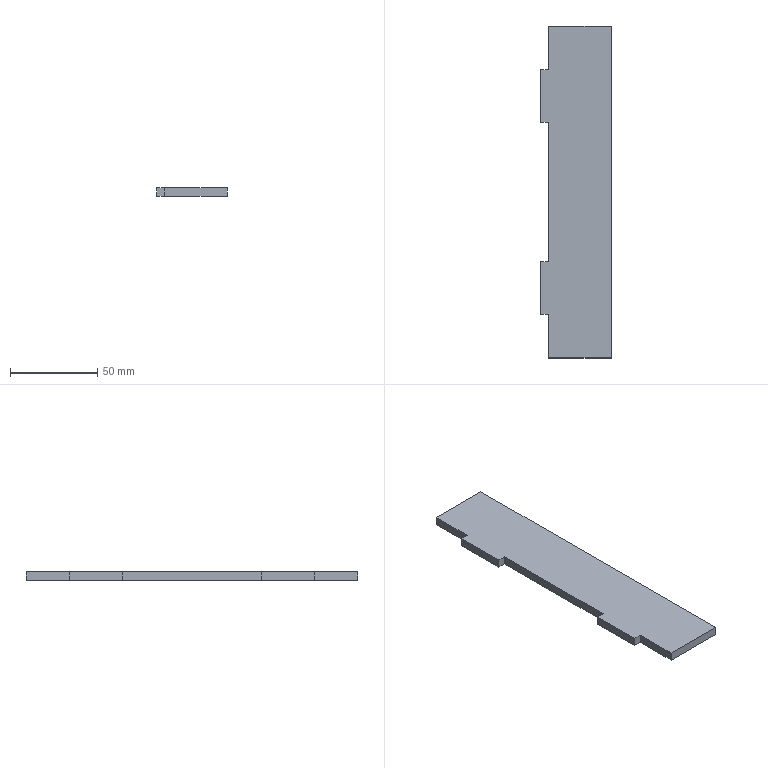Part | SolidWorks | features FlatPattern 1, SMBaseFlange 1, SheetMetal 1 | 1 solid | 14 faces | box 40.5 x 190 x 5 mm | volume 35550 mm3 | plane 14
STEP:
#1=CARTESIAN_POINT('',(-126.05,-77.454,0.));
#2=VERTEX_POINT('',#1);
#3=CARTESIAN_POINT('',(-126.05,-102.454,0.));
#4=VERTEX_POINT('',#3);
#5=CARTESIAN_POINT('',(-126.05,-102.454,0.));
#6=DIRECTION('',(0.,-1.,0.));
#7=VECTOR('',#6,1000.);
#8=LINE('',#5,#7);
#9=EDGE_CURVE('',#2,#4,#8,.T.);
#10=ORIENTED_EDGE('',*,*,#9,.F.);
#11=CARTESIAN_POINT('',(-126.05,-77.454,-5.));
#12=VERTEX_POINT('',#11);
#13=CARTESIAN_POINT('',(-126.05,-77.454,-5.));
#14=DIRECTION('',(0.,0.,1.));
#15=VECTOR('',#14,1000.);
#16=LINE('',#13,#15);
#17=EDGE_CURVE('',#12,#2,#16,.T.);
#18=ORIENTED_EDGE('',*,*,#17,.F.);
#19=CARTESIAN_POINT('',(-126.05,-102.454,-5.));
#20=VERTEX_POINT('',#19);
#21=CARTESIAN_POINT('',(-126.05,-102.454,-5.));
#22=DIRECTION('',(0.,-1.,0.));
#23=VECTOR('',#22,1000.);
#24=LINE('',#21,#23);
#25=EDGE_CURVE('',#12,#20,#24,.T.);
#26=ORIENTED_EDGE('',*,*,#25,.T.);
#27=CARTESIAN_POINT('',(-126.05,-102.454,-5.));
#28=DIRECTION('',(0.,0.,1.));
#29=VECTOR('',#28,1000.);
#30=LINE('',#27,#29);
#31=EDGE_CURVE('',#20,#4,#30,.T.);
#32=ORIENTED_EDGE('',*,*,#31,.T.);
#33=EDGE_LOOP('',(#10,#18,#26,#32));
#34=FACE_OUTER_BOUND('',#33,.T.);
#35=CARTESIAN_POINT('',(-126.05,-102.454,-5.));
#36=DIRECTION('',(-1.,0.,0.));
#37=DIRECTION('',(0.,0.,1.));
#38=AXIS2_PLACEMENT_3D('',#35,#36,#37);
#39=PLANE('',#38);
#40=ADVANCED_FACE('',(#34),#39,.T.);
#41=CARTESIAN_POINT('',(-130.55,-77.454,0.));
#42=VERTEX_POINT('',#41);
#43=CARTESIAN_POINT('',(-126.05,-77.454,0.));
#44=DIRECTION('',(1.,0.,0.));
#45=VECTOR('',#44,1000.);
#46=LINE('',#43,#45);
#47=EDGE_CURVE('',#42,#2,#46,.T.);
#48=ORIENTED_EDGE('',*,*,#47,.F.);
#49=CARTESIAN_POINT('',(-130.55,-77.454,-5.));
#50=VERTEX_POINT('',#49);
#51=CARTESIAN_POINT('',(-130.55,-77.454,-5.));
#52=DIRECTION('',(0.,0.,1.));
#53=VECTOR('',#52,1000.);
#54=LINE('',#51,#53);
#55=EDGE_CURVE('',#50,#42,#54,.T.);
#56=ORIENTED_EDGE('',*,*,#55,.F.);
#57=CARTESIAN_POINT('',(-126.05,-77.454,-5.));
#58=DIRECTION('',(1.,0.,0.));
#59=VECTOR('',#58,1000.);
#60=LINE('',#57,#59);
#61=EDGE_CURVE('',#50,#12,#60,.T.);
#62=ORIENTED_EDGE('',*,*,#61,.T.);
#63=ORIENTED_EDGE('',*,*,#17,.T.);
#64=EDGE_LOOP('',(#48,#56,#62,#63));
#65=FACE_OUTER_BOUND('',#64,.T.);
#66=CARTESIAN_POINT('',(-126.05,-77.454,-5.));
#67=DIRECTION('',(0.,-1.,0.));
#68=DIRECTION('',(0.,0.,-1.));
#69=AXIS2_PLACEMENT_3D('',#66,#67,#68);
#70=PLANE('',#69);
#71=ADVANCED_FACE('',(#65),#70,.T.);
#72=CARTESIAN_POINT('',(-130.55,-47.454,0.));
#73=VERTEX_POINT('',#72);
#74=CARTESIAN_POINT('',(-130.55,-77.454,0.));
#75=DIRECTION('',(0.,-1.,0.));
#76=VECTOR('',#75,1000.);
#77=LINE('',#74,#76);
#78=EDGE_CURVE('',#73,#42,#77,.T.);
#79=ORIENTED_EDGE('',*,*,#78,.F.);
#80=CARTESIAN_POINT('',(-130.55,-47.454,-5.));
#81=VERTEX_POINT('',#80);
#82=CARTESIAN_POINT('',(-130.55,-47.454,-5.));
#83=DIRECTION('',(0.,0.,1.));
#84=VECTOR('',#83,1000.);
#85=LINE('',#82,#84);
#86=EDGE_CURVE('',#81,#73,#85,.T.);
#87=ORIENTED_EDGE('',*,*,#86,.F.);
#88=CARTESIAN_POINT('',(-130.55,-77.454,-5.));
#89=DIRECTION('',(0.,-1.,0.));
#90=VECTOR('',#89,1000.);
#91=LINE('',#88,#90);
#92=EDGE_CURVE('',#81,#50,#91,.T.);
#93=ORIENTED_EDGE('',*,*,#92,.T.);
#94=ORIENTED_EDGE('',*,*,#55,.T.);
#95=EDGE_LOOP('',(#79,#87,#93,#94));
#96=FACE_OUTER_BOUND('',#95,.T.);
#97=CARTESIAN_POINT('',(-130.55,-77.454,-5.));
#98=DIRECTION('',(-1.,0.,0.));
#99=DIRECTION('',(0.,0.,1.));
#100=AXIS2_PLACEMENT_3D('',#97,#98,#99);
#101=PLANE('',#100);
#102=ADVANCED_FACE('',(#96),#101,.T.);
#103=CARTESIAN_POINT('',(-126.05,-47.454,0.));
#104=VERTEX_POINT('',#103);
#105=CARTESIAN_POINT('',(-130.55,-47.454,0.));
#106=DIRECTION('',(-1.,0.,0.));
#107=VECTOR('',#106,1000.);
#108=LINE('',#105,#107);
#109=EDGE_CURVE('',#104,#73,#108,.T.);
#110=ORIENTED_EDGE('',*,*,#109,.F.);
#111=CARTESIAN_POINT('',(-126.05,-47.454,-5.));
#112=VERTEX_POINT('',#111);
#113=CARTESIAN_POINT('',(-126.05,-47.454,-5.));
#114=DIRECTION('',(0.,0.,1.));
#115=VECTOR('',#114,1000.);
#116=LINE('',#113,#115);
#117=EDGE_CURVE('',#112,#104,#116,.T.);
#118=ORIENTED_EDGE('',*,*,#117,.F.);
#119=CARTESIAN_POINT('',(-130.55,-47.454,-5.));
#120=DIRECTION('',(-1.,0.,0.));
#121=VECTOR('',#120,1000.);
#122=LINE('',#119,#121);
#123=EDGE_CURVE('',#112,#81,#122,.T.);
#124=ORIENTED_EDGE('',*,*,#123,.T.);
#125=ORIENTED_EDGE('',*,*,#86,.T.);
#126=EDGE_LOOP('',(#110,#118,#124,#125));
#127=FACE_OUTER_BOUND('',#126,.T.);
#128=CARTESIAN_POINT('',(-130.55,-47.454,-5.));
#129=DIRECTION('',(0.,1.,0.));
#130=DIRECTION('',(0.,0.,1.));
#131=AXIS2_PLACEMENT_3D('',#128,#129,#130);
#132=PLANE('',#131);
#133=ADVANCED_FACE('',(#127),#132,.T.);
#134=CARTESIAN_POINT('',(-126.05,32.546,0.));
#135=VERTEX_POINT('',#134);
#136=CARTESIAN_POINT('',(-126.05,-47.454,0.));
#137=DIRECTION('',(0.,-1.,0.));
#138=VECTOR('',#137,1000.);
#139=LINE('',#136,#138);
#140=EDGE_CURVE('',#135,#104,#139,.T.);
#141=ORIENTED_EDGE('',*,*,#140,.F.);
#142=CARTESIAN_POINT('',(-126.05,32.546,-5.));
#143=VERTEX_POINT('',#142);
#144=CARTESIAN_POINT('',(-126.05,32.546,-5.));
#145=DIRECTION('',(0.,0.,1.));
#146=VECTOR('',#145,1000.);
#147=LINE('',#144,#146);
#148=EDGE_CURVE('',#143,#135,#147,.T.);
#149=ORIENTED_EDGE('',*,*,#148,.F.);
#150=CARTESIAN_POINT('',(-126.05,-47.454,-5.));
#151=DIRECTION('',(0.,-1.,0.));
#152=VECTOR('',#151,1000.);
#153=LINE('',#150,#152);
#154=EDGE_CURVE('',#143,#112,#153,.T.);
#155=ORIENTED_EDGE('',*,*,#154,.T.);
#156=ORIENTED_EDGE('',*,*,#117,.T.);
#157=EDGE_LOOP('',(#141,#149,#155,#156));
#158=FACE_OUTER_BOUND('',#157,.T.);
#159=CARTESIAN_POINT('',(-126.05,-47.454,-5.));
#160=DIRECTION('',(-1.,0.,0.));
#161=DIRECTION('',(0.,0.,1.));
#162=AXIS2_PLACEMENT_3D('',#159,#160,#161);
#163=PLANE('',#162);
#164=ADVANCED_FACE('',(#158),#163,.T.);
#165=CARTESIAN_POINT('',(-130.55,32.546,0.));
#166=VERTEX_POINT('',#165);
#167=CARTESIAN_POINT('',(-130.55,32.546,0.));
#168=DIRECTION('',(1.,0.,0.));
#169=VECTOR('',#168,1000.);
#170=LINE('',#167,#169);
#171=EDGE_CURVE('',#166,#135,#170,.T.);
#172=ORIENTED_EDGE('',*,*,#171,.F.);
#173=CARTESIAN_POINT('',(-130.55,32.546,-5.));
#174=VERTEX_POINT('',#173);
#175=CARTESIAN_POINT('',(-130.55,32.546,-5.));
#176=DIRECTION('',(0.,0.,1.));
#177=VECTOR('',#176,1000.);
#178=LINE('',#175,#177);
#179=EDGE_CURVE('',#174,#166,#178,.T.);
#180=ORIENTED_EDGE('',*,*,#179,.F.);
#181=CARTESIAN_POINT('',(-130.55,32.546,-5.));
#182=DIRECTION('',(1.,0.,0.));
#183=VECTOR('',#182,1000.);
#184=LINE('',#181,#183);
#185=EDGE_CURVE('',#174,#143,#184,.T.);
#186=ORIENTED_EDGE('',*,*,#185,.T.);
#187=ORIENTED_EDGE('',*,*,#148,.T.);
#188=EDGE_LOOP('',(#172,#180,#186,#187));
#189=FACE_OUTER_BOUND('',#188,.T.);
#190=CARTESIAN_POINT('',(-130.55,32.546,-5.));
#191=DIRECTION('',(0.,-1.,0.));
#192=DIRECTION('',(0.,0.,-1.));
#193=AXIS2_PLACEMENT_3D('',#190,#191,#192);
#194=PLANE('',#193);
#195=ADVANCED_FACE('',(#189),#194,.T.);
#196=CARTESIAN_POINT('',(-130.55,62.546,0.));
#197=VERTEX_POINT('',#196);
#198=CARTESIAN_POINT('',(-130.55,62.546,0.));
#199=DIRECTION('',(0.,-1.,0.));
#200=VECTOR('',#199,1000.);
#201=LINE('',#198,#200);
#202=EDGE_CURVE('',#197,#166,#201,.T.);
#203=ORIENTED_EDGE('',*,*,#202,.F.);
#204=CARTESIAN_POINT('',(-130.55,62.546,-5.));
#205=VERTEX_POINT('',#204);
#206=CARTESIAN_POINT('',(-130.55,62.546,-5.));
#207=DIRECTION('',(0.,0.,1.));
#208=VECTOR('',#207,1000.);
#209=LINE('',#206,#208);
#210=EDGE_CURVE('',#205,#197,#209,.T.);
#211=ORIENTED_EDGE('',*,*,#210,.F.);
#212=CARTESIAN_POINT('',(-130.55,62.546,-5.));
#213=DIRECTION('',(0.,-1.,0.));
#214=VECTOR('',#213,1000.);
#215=LINE('',#212,#214);
#216=EDGE_CURVE('',#205,#174,#215,.T.);
#217=ORIENTED_EDGE('',*,*,#216,.T.);
#218=ORIENTED_EDGE('',*,*,#179,.T.);
#219=EDGE_LOOP('',(#203,#211,#217,#218));
#220=FACE_OUTER_BOUND('',#219,.T.);
#221=CARTESIAN_POINT('',(-130.55,62.546,-5.));
#222=DIRECTION('',(-1.,0.,0.));
#223=DIRECTION('',(0.,-1.,0.));
#224=AXIS2_PLACEMENT_3D('',#221,#222,#223);
#225=PLANE('',#224);
#226=ADVANCED_FACE('',(#220),#225,.T.);
#227=CARTESIAN_POINT('',(-126.05,62.546,0.));
#228=VERTEX_POINT('',#227);
#229=CARTESIAN_POINT('',(-126.05,62.546,0.));
#230=DIRECTION('',(-1.,0.,0.));
#231=VECTOR('',#230,1000.);
#232=LINE('',#229,#231);
#233=EDGE_CURVE('',#228,#197,#232,.T.);
#234=ORIENTED_EDGE('',*,*,#233,.F.);
#235=CARTESIAN_POINT('',(-126.05,62.546,-5.));
#236=VERTEX_POINT('',#235);
#237=CARTESIAN_POINT('',(-126.05,62.546,-5.));
#238=DIRECTION('',(0.,0.,1.));
#239=VECTOR('',#238,1000.);
#240=LINE('',#237,#239);
#241=EDGE_CURVE('',#236,#228,#240,.T.);
#242=ORIENTED_EDGE('',*,*,#241,.F.);
#243=CARTESIAN_POINT('',(-126.05,62.546,-5.));
#244=DIRECTION('',(-1.,0.,0.));
#245=VECTOR('',#244,1000.);
#246=LINE('',#243,#245);
#247=EDGE_CURVE('',#236,#205,#246,.T.);
#248=ORIENTED_EDGE('',*,*,#247,.T.);
#249=ORIENTED_EDGE('',*,*,#210,.T.);
#250=EDGE_LOOP('',(#234,#242,#248,#249));
#251=FACE_OUTER_BOUND('',#250,.T.);
#252=CARTESIAN_POINT('',(-126.05,62.546,-5.));
#253=DIRECTION('',(0.,1.,0.));
#254=DIRECTION('',(0.,0.,1.));
#255=AXIS2_PLACEMENT_3D('',#252,#253,#254);
#256=PLANE('',#255);
#257=ADVANCED_FACE('',(#251),#256,.T.);
#258=CARTESIAN_POINT('',(-126.05,87.546,0.));
#259=VERTEX_POINT('',#258);
#260=CARTESIAN_POINT('',(-126.05,62.546,0.));
#261=DIRECTION('',(0.,-1.,0.));
#262=VECTOR('',#261,1000.);
#263=LINE('',#260,#262);
#264=EDGE_CURVE('',#259,#228,#263,.T.);
#265=ORIENTED_EDGE('',*,*,#264,.F.);
#266=CARTESIAN_POINT('',(-126.05,87.546,-5.));
#267=VERTEX_POINT('',#266);
#268=CARTESIAN_POINT('',(-126.05,87.546,-5.));
#269=DIRECTION('',(0.,0.,1.));
#270=VECTOR('',#269,1000.);
#271=LINE('',#268,#270);
#272=EDGE_CURVE('',#267,#259,#271,.T.);
#273=ORIENTED_EDGE('',*,*,#272,.F.);
#274=CARTESIAN_POINT('',(-126.05,62.546,-5.));
#275=DIRECTION('',(0.,-1.,0.));
#276=VECTOR('',#275,1000.);
#277=LINE('',#274,#276);
#278=EDGE_CURVE('',#267,#236,#277,.T.);
#279=ORIENTED_EDGE('',*,*,#278,.T.);
#280=ORIENTED_EDGE('',*,*,#241,.T.);
#281=EDGE_LOOP('',(#265,#273,#279,#280));
#282=FACE_OUTER_BOUND('',#281,.T.);
#283=CARTESIAN_POINT('',(-126.05,62.546,-5.));
#284=DIRECTION('',(-1.,0.,0.));
#285=DIRECTION('',(0.,0.,1.));
#286=AXIS2_PLACEMENT_3D('',#283,#284,#285);
#287=PLANE('',#286);
#288=ADVANCED_FACE('',(#282),#287,.T.);
#289=CARTESIAN_POINT('',(-90.05,87.546,0.));
#290=VERTEX_POINT('',#289);
#291=CARTESIAN_POINT('',(-126.05,87.546,0.));
#292=DIRECTION('',(-1.,0.,0.));
#293=VECTOR('',#292,1000.);
#294=LINE('',#291,#293);
#295=EDGE_CURVE('',#290,#259,#294,.T.);
#296=ORIENTED_EDGE('',*,*,#295,.F.);
#297=CARTESIAN_POINT('',(-90.05,87.546,-5.));
#298=VERTEX_POINT('',#297);
#299=CARTESIAN_POINT('',(-90.05,87.546,-5.));
#300=DIRECTION('',(0.,0.,1.));
#301=VECTOR('',#300,1000.);
#302=LINE('',#299,#301);
#303=EDGE_CURVE('',#298,#290,#302,.T.);
#304=ORIENTED_EDGE('',*,*,#303,.F.);
#305=CARTESIAN_POINT('',(-126.05,87.546,-5.));
#306=DIRECTION('',(-1.,0.,0.));
#307=VECTOR('',#306,1000.);
#308=LINE('',#305,#307);
#309=EDGE_CURVE('',#298,#267,#308,.T.);
#310=ORIENTED_EDGE('',*,*,#309,.T.);
#311=ORIENTED_EDGE('',*,*,#272,.T.);
#312=EDGE_LOOP('',(#296,#304,#310,#311));
#313=FACE_OUTER_BOUND('',#312,.T.);
#314=CARTESIAN_POINT('',(-126.05,87.546,-5.));
#315=DIRECTION('',(0.,1.,0.));
#316=DIRECTION('',(0.,0.,1.));
#317=AXIS2_PLACEMENT_3D('',#314,#315,#316);
#318=PLANE('',#317);
#319=ADVANCED_FACE('',(#313),#318,.T.);
#320=CARTESIAN_POINT('',(-90.05,-102.454,0.));
#321=VERTEX_POINT('',#320);
#322=CARTESIAN_POINT('',(-90.05,-102.454,0.));
#323=DIRECTION('',(0.,1.,0.));
#324=VECTOR('',#323,1000.);
#325=LINE('',#322,#324);
#326=EDGE_CURVE('',#321,#290,#325,.T.);
#327=ORIENTED_EDGE('',*,*,#326,.F.);
#328=CARTESIAN_POINT('',(-90.05,-102.454,-5.));
#329=VERTEX_POINT('',#328);
#330=CARTESIAN_POINT('',(-90.05,-102.454,-5.));
#331=DIRECTION('',(0.,0.,1.));
#332=VECTOR('',#331,1000.);
#333=LINE('',#330,#332);
#334=EDGE_CURVE('',#329,#321,#333,.T.);
#335=ORIENTED_EDGE('',*,*,#334,.F.);
#336=CARTESIAN_POINT('',(-90.05,-102.454,-5.));
#337=DIRECTION('',(0.,1.,0.));
#338=VECTOR('',#337,1000.);
#339=LINE('',#336,#338);
#340=EDGE_CURVE('',#329,#298,#339,.T.);
#341=ORIENTED_EDGE('',*,*,#340,.T.);
#342=ORIENTED_EDGE('',*,*,#303,.T.);
#343=EDGE_LOOP('',(#327,#335,#341,#342));
#344=FACE_OUTER_BOUND('',#343,.T.);
#345=CARTESIAN_POINT('',(-90.05,-102.454,-5.));
#346=DIRECTION('',(1.,0.,0.));
#347=DIRECTION('',(0.,0.,-1.));
#348=AXIS2_PLACEMENT_3D('',#345,#346,#347);
#349=PLANE('',#348);
#350=ADVANCED_FACE('',(#344),#349,.T.);
#351=CARTESIAN_POINT('',(-126.05,-102.454,0.));
#352=DIRECTION('',(1.,0.,0.));
#353=VECTOR('',#352,1000.);
#354=LINE('',#351,#353);
#355=EDGE_CURVE('',#4,#321,#354,.T.);
#356=ORIENTED_EDGE('',*,*,#355,.F.);
#357=ORIENTED_EDGE('',*,*,#31,.F.);
#358=CARTESIAN_POINT('',(-126.05,-102.454,-5.));
#359=DIRECTION('',(1.,0.,0.));
#360=VECTOR('',#359,1000.);
#361=LINE('',#358,#360);
#362=EDGE_CURVE('',#20,#329,#361,.T.);
#363=ORIENTED_EDGE('',*,*,#362,.T.);
#364=ORIENTED_EDGE('',*,*,#334,.T.);
#365=EDGE_LOOP('',(#356,#357,#363,#364));
#366=FACE_OUTER_BOUND('',#365,.T.);
#367=CARTESIAN_POINT('',(-126.05,-102.454,-5.));
#368=DIRECTION('',(0.,-1.,0.));
#369=DIRECTION('',(0.,0.,-1.));
#370=AXIS2_PLACEMENT_3D('',#367,#368,#369);
#371=PLANE('',#370);
#372=ADVANCED_FACE('',(#366),#371,.T.);
#373=ORIENTED_EDGE('',*,*,#25,.F.);
#374=ORIENTED_EDGE('',*,*,#61,.F.);
#375=ORIENTED_EDGE('',*,*,#92,.F.);
#376=ORIENTED_EDGE('',*,*,#123,.F.);
#377=ORIENTED_EDGE('',*,*,#154,.F.);
#378=ORIENTED_EDGE('',*,*,#185,.F.);
#379=ORIENTED_EDGE('',*,*,#216,.F.);
#380=ORIENTED_EDGE('',*,*,#247,.F.);
#381=ORIENTED_EDGE('',*,*,#278,.F.);
#382=ORIENTED_EDGE('',*,*,#309,.F.);
#383=ORIENTED_EDGE('',*,*,#340,.F.);
#384=ORIENTED_EDGE('',*,*,#362,.F.);
#385=EDGE_LOOP('',(#373,#374,#375,#376,#377,#378,#379,#380,#381,#382,#383,#384));
#386=FACE_OUTER_BOUND('',#385,.T.);
#387=CARTESIAN_POINT('',(0.,0.,-5.));
#388=DIRECTION('',(0.,0.,1.));
#389=DIRECTION('',(1.,0.,0.));
#390=AXIS2_PLACEMENT_3D('',#387,#388,#389);
#391=PLANE('',#390);
#392=ADVANCED_FACE('',(#386),#391,.F.);
#393=ORIENTED_EDGE('',*,*,#9,.T.);
#394=ORIENTED_EDGE('',*,*,#355,.T.);
#395=ORIENTED_EDGE('',*,*,#326,.T.);
#396=ORIENTED_EDGE('',*,*,#295,.T.);
#397=ORIENTED_EDGE('',*,*,#264,.T.);
#398=ORIENTED_EDGE('',*,*,#233,.T.);
#399=ORIENTED_EDGE('',*,*,#202,.T.);
#400=ORIENTED_EDGE('',*,*,#171,.T.);
#401=ORIENTED_EDGE('',*,*,#140,.T.);
#402=ORIENTED_EDGE('',*,*,#109,.T.);
#403=ORIENTED_EDGE('',*,*,#78,.T.);
#404=ORIENTED_EDGE('',*,*,#47,.T.);
#405=EDGE_LOOP('',(#393,#394,#395,#396,#397,#398,#399,#400,#401,#402,#403,#404));
#406=FACE_OUTER_BOUND('',#405,.T.);
#407=CARTESIAN_POINT('',(0.,0.,0.));
#408=DIRECTION('',(0.,0.,1.));
#409=DIRECTION('',(1.,0.,0.));
#410=AXIS2_PLACEMENT_3D('',#407,#408,#409);
#411=PLANE('',#410);
#412=ADVANCED_FACE('',(#406),#411,.T.);
#413=CLOSED_SHELL('',(#40,#71,#102,#133,#164,#195,#226,#257,#288,#319,#350,#372,#392,#412));
#414=MANIFOLD_SOLID_BREP('',#413);
#415=CARTESIAN_POINT('',(0.,0.,0.));
#416=DIRECTION('',(0.,0.,1.));
#417=DIRECTION('',(1.,0.,0.));
#418=AXIS2_PLACEMENT_3D('',#415,#416,#417);
#419=(LENGTH_UNIT()NAMED_UNIT(*)SI_UNIT(.MILLI.,.METRE.));
#420=UNCERTAINTY_MEASURE_WITH_UNIT(LENGTH_MEASURE(0.00001),#419,'','');
#421=(NAMED_UNIT(*)PLANE_ANGLE_UNIT()SI_UNIT($,.RADIAN.));
#422=(NAMED_UNIT(*)SI_UNIT($,.STERADIAN.)SOLID_ANGLE_UNIT());
#423=(GEOMETRIC_REPRESENTATION_CONTEXT(3)GLOBAL_UNCERTAINTY_ASSIGNED_CONTEXT((#420))GLOBAL_UNIT_ASSIGNED_CONTEXT((#419,#421,#422))REPRESENTATION_CONTEXT('',''));
#424=ADVANCED_BREP_SHAPE_REPRESENTATION('',(#414,#418),#423);